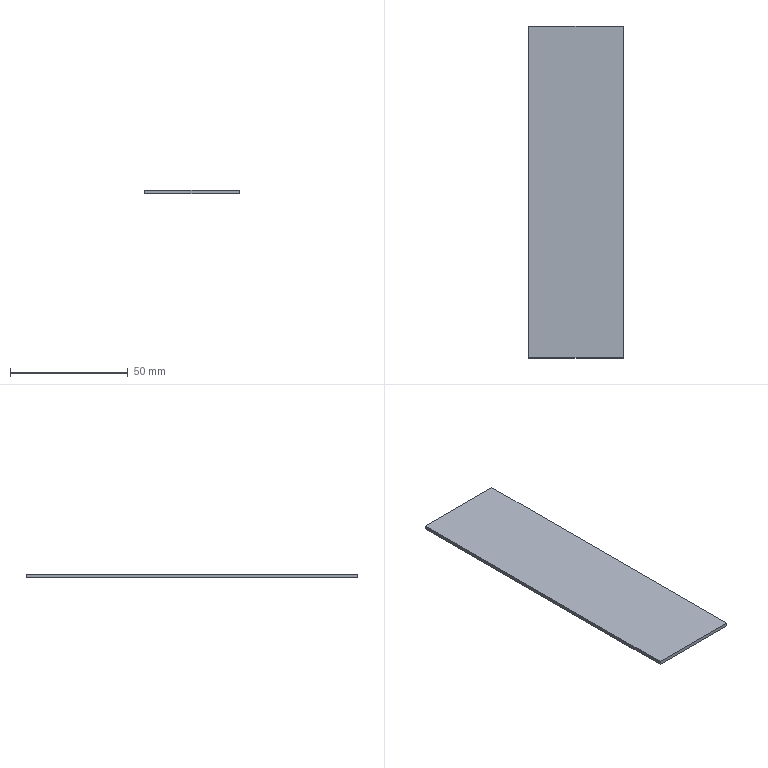Part | 1 solid | 6 faces | box 40 x 141 x 1.5 mm | volume 8460 mm3 | plane 6
STEP:
#1=CARTESIAN_POINT('',(20.,-70.5,0.));
#2=VERTEX_POINT('',#1);
#3=CARTESIAN_POINT('',(20.,70.5,0.));
#4=VERTEX_POINT('',#3);
#5=CARTESIAN_POINT('',(20.,-70.5,0.));
#6=DIRECTION('',(0.,1.,0.));
#7=VECTOR('',#6,1000.);
#8=LINE('',#5,#7);
#9=EDGE_CURVE('',#2,#4,#8,.T.);
#10=ORIENTED_EDGE('',*,*,#9,.F.);
#11=CARTESIAN_POINT('',(20.,-70.5,-1.5));
#12=VERTEX_POINT('',#11);
#13=CARTESIAN_POINT('',(20.,-70.5,-1.5));
#14=DIRECTION('',(0.,0.,1.));
#15=VECTOR('',#14,1000.);
#16=LINE('',#13,#15);
#17=EDGE_CURVE('',#12,#2,#16,.T.);
#18=ORIENTED_EDGE('',*,*,#17,.F.);
#19=CARTESIAN_POINT('',(20.,70.5,-1.5));
#20=VERTEX_POINT('',#19);
#21=CARTESIAN_POINT('',(20.,-70.5,-1.5));
#22=DIRECTION('',(0.,1.,0.));
#23=VECTOR('',#22,1000.);
#24=LINE('',#21,#23);
#25=EDGE_CURVE('',#12,#20,#24,.T.);
#26=ORIENTED_EDGE('',*,*,#25,.T.);
#27=CARTESIAN_POINT('',(20.,70.5,-1.5));
#28=DIRECTION('',(0.,0.,1.));
#29=VECTOR('',#28,1000.);
#30=LINE('',#27,#29);
#31=EDGE_CURVE('',#20,#4,#30,.T.);
#32=ORIENTED_EDGE('',*,*,#31,.T.);
#33=EDGE_LOOP('',(#10,#18,#26,#32));
#34=FACE_OUTER_BOUND('',#33,.T.);
#35=CARTESIAN_POINT('',(20.,-70.5,-1.5));
#36=DIRECTION('',(1.,0.,0.));
#37=DIRECTION('',(0.,0.,-1.));
#38=AXIS2_PLACEMENT_3D('',#35,#36,#37);
#39=PLANE('',#38);
#40=ADVANCED_FACE('',(#34),#39,.T.);
#41=CARTESIAN_POINT('',(-20.,-70.5,0.));
#42=VERTEX_POINT('',#41);
#43=CARTESIAN_POINT('',(-20.,-70.5,0.));
#44=DIRECTION('',(1.,0.,0.));
#45=VECTOR('',#44,1000.);
#46=LINE('',#43,#45);
#47=EDGE_CURVE('',#42,#2,#46,.T.);
#48=ORIENTED_EDGE('',*,*,#47,.F.);
#49=CARTESIAN_POINT('',(-20.,-70.5,-1.5));
#50=VERTEX_POINT('',#49);
#51=CARTESIAN_POINT('',(-20.,-70.5,-1.5));
#52=DIRECTION('',(0.,0.,1.));
#53=VECTOR('',#52,1000.);
#54=LINE('',#51,#53);
#55=EDGE_CURVE('',#50,#42,#54,.T.);
#56=ORIENTED_EDGE('',*,*,#55,.F.);
#57=CARTESIAN_POINT('',(-20.,-70.5,-1.5));
#58=DIRECTION('',(1.,0.,0.));
#59=VECTOR('',#58,1000.);
#60=LINE('',#57,#59);
#61=EDGE_CURVE('',#50,#12,#60,.T.);
#62=ORIENTED_EDGE('',*,*,#61,.T.);
#63=ORIENTED_EDGE('',*,*,#17,.T.);
#64=EDGE_LOOP('',(#48,#56,#62,#63));
#65=FACE_OUTER_BOUND('',#64,.T.);
#66=CARTESIAN_POINT('',(-20.,-70.5,-1.5));
#67=DIRECTION('',(0.,-1.,0.));
#68=DIRECTION('',(0.,0.,-1.));
#69=AXIS2_PLACEMENT_3D('',#66,#67,#68);
#70=PLANE('',#69);
#71=ADVANCED_FACE('',(#65),#70,.T.);
#72=CARTESIAN_POINT('',(-20.,70.5,0.));
#73=VERTEX_POINT('',#72);
#74=CARTESIAN_POINT('',(-20.,-70.5,0.));
#75=DIRECTION('',(0.,-1.,0.));
#76=VECTOR('',#75,1000.);
#77=LINE('',#74,#76);
#78=EDGE_CURVE('',#73,#42,#77,.T.);
#79=ORIENTED_EDGE('',*,*,#78,.F.);
#80=CARTESIAN_POINT('',(-20.,70.5,-1.5));
#81=VERTEX_POINT('',#80);
#82=CARTESIAN_POINT('',(-20.,70.5,-1.5));
#83=DIRECTION('',(0.,0.,1.));
#84=VECTOR('',#83,1000.);
#85=LINE('',#82,#84);
#86=EDGE_CURVE('',#81,#73,#85,.T.);
#87=ORIENTED_EDGE('',*,*,#86,.F.);
#88=CARTESIAN_POINT('',(-20.,-70.5,-1.5));
#89=DIRECTION('',(0.,-1.,0.));
#90=VECTOR('',#89,1000.);
#91=LINE('',#88,#90);
#92=EDGE_CURVE('',#81,#50,#91,.T.);
#93=ORIENTED_EDGE('',*,*,#92,.T.);
#94=ORIENTED_EDGE('',*,*,#55,.T.);
#95=EDGE_LOOP('',(#79,#87,#93,#94));
#96=FACE_OUTER_BOUND('',#95,.T.);
#97=CARTESIAN_POINT('',(-20.,-70.5,-1.5));
#98=DIRECTION('',(-1.,0.,0.));
#99=DIRECTION('',(0.,0.,1.));
#100=AXIS2_PLACEMENT_3D('',#97,#98,#99);
#101=PLANE('',#100);
#102=ADVANCED_FACE('',(#96),#101,.T.);
#103=CARTESIAN_POINT('',(-20.,70.5,0.));
#104=DIRECTION('',(-1.,0.,0.));
#105=VECTOR('',#104,1000.);
#106=LINE('',#103,#105);
#107=EDGE_CURVE('',#4,#73,#106,.T.);
#108=ORIENTED_EDGE('',*,*,#107,.F.);
#109=ORIENTED_EDGE('',*,*,#31,.F.);
#110=CARTESIAN_POINT('',(-20.,70.5,-1.5));
#111=DIRECTION('',(-1.,0.,0.));
#112=VECTOR('',#111,1000.);
#113=LINE('',#110,#112);
#114=EDGE_CURVE('',#20,#81,#113,.T.);
#115=ORIENTED_EDGE('',*,*,#114,.T.);
#116=ORIENTED_EDGE('',*,*,#86,.T.);
#117=EDGE_LOOP('',(#108,#109,#115,#116));
#118=FACE_OUTER_BOUND('',#117,.T.);
#119=CARTESIAN_POINT('',(-20.,70.5,-1.5));
#120=DIRECTION('',(0.,1.,0.));
#121=DIRECTION('',(0.,0.,1.));
#122=AXIS2_PLACEMENT_3D('',#119,#120,#121);
#123=PLANE('',#122);
#124=ADVANCED_FACE('',(#118),#123,.T.);
#125=ORIENTED_EDGE('',*,*,#25,.F.);
#126=ORIENTED_EDGE('',*,*,#61,.F.);
#127=ORIENTED_EDGE('',*,*,#92,.F.);
#128=ORIENTED_EDGE('',*,*,#114,.F.);
#129=EDGE_LOOP('',(#125,#126,#127,#128));
#130=FACE_OUTER_BOUND('',#129,.T.);
#131=CARTESIAN_POINT('',(0.,0.,-1.5));
#132=DIRECTION('',(0.,0.,-1.));
#133=DIRECTION('',(-1.,0.,0.));
#134=AXIS2_PLACEMENT_3D('',#131,#132,#133);
#135=PLANE('',#134);
#136=ADVANCED_FACE('',(#130),#135,.T.);
#137=ORIENTED_EDGE('',*,*,#9,.T.);
#138=ORIENTED_EDGE('',*,*,#107,.T.);
#139=ORIENTED_EDGE('',*,*,#78,.T.);
#140=ORIENTED_EDGE('',*,*,#47,.T.);
#141=EDGE_LOOP('',(#137,#138,#139,#140));
#142=FACE_OUTER_BOUND('',#141,.T.);
#143=CARTESIAN_POINT('',(0.,0.,0.));
#144=DIRECTION('',(0.,0.,-1.));
#145=DIRECTION('',(-1.,0.,0.));
#146=AXIS2_PLACEMENT_3D('',#143,#144,#145);
#147=PLANE('',#146);
#148=ADVANCED_FACE('',(#142),#147,.F.);
#149=CLOSED_SHELL('',(#40,#71,#102,#124,#136,#148));
#150=MANIFOLD_SOLID_BREP('',#149);
#151=CARTESIAN_POINT('',(0.,0.,0.));
#152=DIRECTION('',(0.,0.,1.));
#153=DIRECTION('',(1.,0.,0.));
#154=AXIS2_PLACEMENT_3D('',#151,#152,#153);
#155=(LENGTH_UNIT()NAMED_UNIT(*)SI_UNIT(.MILLI.,.METRE.));
#156=UNCERTAINTY_MEASURE_WITH_UNIT(LENGTH_MEASURE(0.00001),#155,'','');
#157=(NAMED_UNIT(*)PLANE_ANGLE_UNIT()SI_UNIT($,.RADIAN.));
#158=(NAMED_UNIT(*)SI_UNIT($,.STERADIAN.)SOLID_ANGLE_UNIT());
#159=(GEOMETRIC_REPRESENTATION_CONTEXT(3)GLOBAL_UNCERTAINTY_ASSIGNED_CONTEXT((#156))GLOBAL_UNIT_ASSIGNED_CONTEXT((#155,#157,#158))REPRESENTATION_CONTEXT('',''));
#160=ADVANCED_BREP_SHAPE_REPRESENTATION('',(#150,#154),#159);